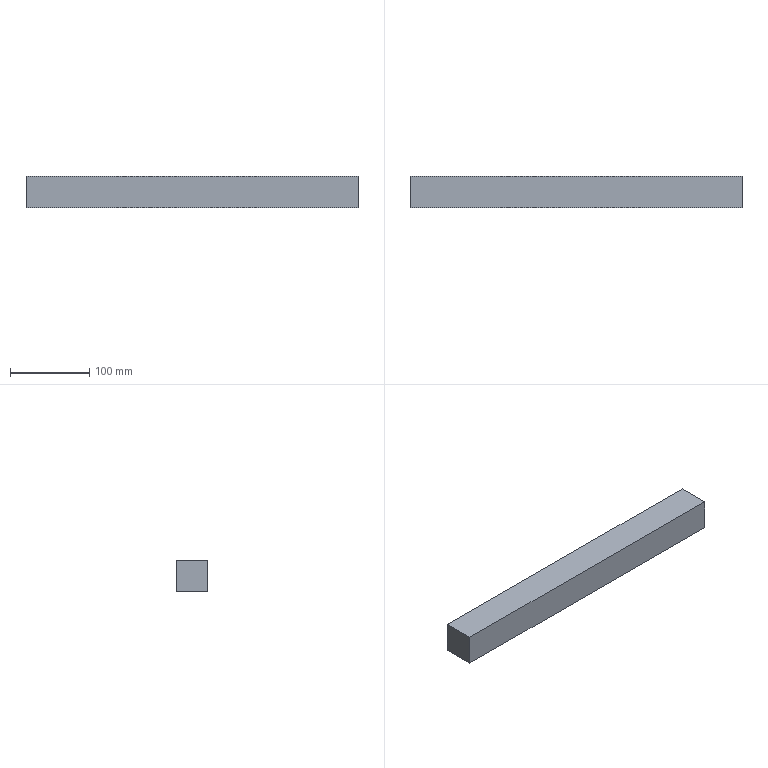Part | NX | 1 solid | 6 faces | box 420 x 40 x 40 mm | volume 672000 mm3 | plane 6
STEP:
#1=CARTESIAN_POINT('',(-369.726,88.985,0.));
#2=VERTEX_POINT('',#1);
#3=CARTESIAN_POINT('',(-369.726,88.985,-40.));
#4=VERTEX_POINT('',#3);
#5=CARTESIAN_POINT('',(-369.726,88.985,0.));
#6=DIRECTION('',(0.,0.,-1.));
#7=VECTOR('',#6,1000.);
#8=LINE('',#5,#7);
#9=EDGE_CURVE('',#2,#4,#8,.T.);
#10=ORIENTED_EDGE('',*,*,#9,.F.);
#11=CARTESIAN_POINT('',(50.274,88.985,0.));
#12=VERTEX_POINT('',#11);
#13=CARTESIAN_POINT('',(-369.726,88.985,0.));
#14=DIRECTION('',(1.,0.,0.));
#15=VECTOR('',#14,1000.);
#16=LINE('',#13,#15);
#17=EDGE_CURVE('',#2,#12,#16,.T.);
#18=ORIENTED_EDGE('',*,*,#17,.T.);
#19=CARTESIAN_POINT('',(50.274,88.985,-40.));
#20=VERTEX_POINT('',#19);
#21=CARTESIAN_POINT('',(50.274,88.985,0.));
#22=DIRECTION('',(0.,0.,-1.));
#23=VECTOR('',#22,1000.);
#24=LINE('',#21,#23);
#25=EDGE_CURVE('',#12,#20,#24,.T.);
#26=ORIENTED_EDGE('',*,*,#25,.T.);
#27=CARTESIAN_POINT('',(-369.726,88.985,-40.));
#28=DIRECTION('',(1.,0.,0.));
#29=VECTOR('',#28,1000.);
#30=LINE('',#27,#29);
#31=EDGE_CURVE('',#4,#20,#30,.T.);
#32=ORIENTED_EDGE('',*,*,#31,.F.);
#33=EDGE_LOOP('',(#10,#18,#26,#32));
#34=FACE_BOUND('',#33,.T.);
#35=CARTESIAN_POINT('',(-369.726,88.985,0.));
#36=DIRECTION('',(0.,1.,0.));
#37=DIRECTION('',(1.,0.,0.));
#38=AXIS2_PLACEMENT_3D('',#35,#36,#37);
#39=PLANE('',#38);
#40=ADVANCED_FACE('',(#34),#39,.T.);
#41=CARTESIAN_POINT('',(-369.726,48.985,0.));
#42=VERTEX_POINT('',#41);
#43=CARTESIAN_POINT('',(-369.726,88.985,0.));
#44=DIRECTION('',(0.,-1.,0.));
#45=VECTOR('',#44,1000.);
#46=LINE('',#43,#45);
#47=EDGE_CURVE('',#2,#42,#46,.T.);
#48=ORIENTED_EDGE('',*,*,#47,.T.);
#49=CARTESIAN_POINT('',(50.274,48.985,0.));
#50=VERTEX_POINT('',#49);
#51=CARTESIAN_POINT('',(-369.726,48.985,0.));
#52=DIRECTION('',(1.,0.,0.));
#53=VECTOR('',#52,1000.);
#54=LINE('',#51,#53);
#55=EDGE_CURVE('',#42,#50,#54,.T.);
#56=ORIENTED_EDGE('',*,*,#55,.T.);
#57=CARTESIAN_POINT('',(50.274,88.985,0.));
#58=DIRECTION('',(0.,-1.,0.));
#59=VECTOR('',#58,1000.);
#60=LINE('',#57,#59);
#61=EDGE_CURVE('',#12,#50,#60,.T.);
#62=ORIENTED_EDGE('',*,*,#61,.F.);
#63=ORIENTED_EDGE('',*,*,#17,.F.);
#64=EDGE_LOOP('',(#48,#56,#62,#63));
#65=FACE_BOUND('',#64,.T.);
#66=CARTESIAN_POINT('',(-369.726,48.985,0.));
#67=DIRECTION('',(0.,0.,1.));
#68=DIRECTION('',(1.,0.,0.));
#69=AXIS2_PLACEMENT_3D('',#66,#67,#68);
#70=PLANE('',#69);
#71=ADVANCED_FACE('',(#65),#70,.T.);
#72=CARTESIAN_POINT('',(-369.726,48.985,-40.));
#73=VERTEX_POINT('',#72);
#74=CARTESIAN_POINT('',(-369.726,48.985,0.));
#75=DIRECTION('',(0.,0.,-1.));
#76=VECTOR('',#75,1000.);
#77=LINE('',#74,#76);
#78=EDGE_CURVE('',#42,#73,#77,.T.);
#79=ORIENTED_EDGE('',*,*,#78,.T.);
#80=CARTESIAN_POINT('',(50.274,48.985,-40.));
#81=VERTEX_POINT('',#80);
#82=CARTESIAN_POINT('',(-369.726,48.985,-40.));
#83=DIRECTION('',(1.,0.,0.));
#84=VECTOR('',#83,1000.);
#85=LINE('',#82,#84);
#86=EDGE_CURVE('',#73,#81,#85,.T.);
#87=ORIENTED_EDGE('',*,*,#86,.T.);
#88=CARTESIAN_POINT('',(50.274,48.985,0.));
#89=DIRECTION('',(0.,0.,-1.));
#90=VECTOR('',#89,1000.);
#91=LINE('',#88,#90);
#92=EDGE_CURVE('',#50,#81,#91,.T.);
#93=ORIENTED_EDGE('',*,*,#92,.F.);
#94=ORIENTED_EDGE('',*,*,#55,.F.);
#95=EDGE_LOOP('',(#79,#87,#93,#94));
#96=FACE_BOUND('',#95,.T.);
#97=CARTESIAN_POINT('',(-369.726,48.985,-40.));
#98=DIRECTION('',(0.,-1.,0.));
#99=DIRECTION('',(0.,0.,-1.));
#100=AXIS2_PLACEMENT_3D('',#97,#98,#99);
#101=PLANE('',#100);
#102=ADVANCED_FACE('',(#96),#101,.T.);
#103=CARTESIAN_POINT('',(-369.726,88.985,-40.));
#104=DIRECTION('',(0.,-1.,0.));
#105=VECTOR('',#104,1000.);
#106=LINE('',#103,#105);
#107=EDGE_CURVE('',#4,#73,#106,.T.);
#108=ORIENTED_EDGE('',*,*,#107,.F.);
#109=ORIENTED_EDGE('',*,*,#31,.T.);
#110=CARTESIAN_POINT('',(50.274,88.985,-40.));
#111=DIRECTION('',(0.,-1.,0.));
#112=VECTOR('',#111,1000.);
#113=LINE('',#110,#112);
#114=EDGE_CURVE('',#20,#81,#113,.T.);
#115=ORIENTED_EDGE('',*,*,#114,.T.);
#116=ORIENTED_EDGE('',*,*,#86,.F.);
#117=EDGE_LOOP('',(#108,#109,#115,#116));
#118=FACE_BOUND('',#117,.T.);
#119=CARTESIAN_POINT('',(-369.726,88.985,-40.));
#120=DIRECTION('',(0.,0.,-1.));
#121=DIRECTION('',(0.,-1.,0.));
#122=AXIS2_PLACEMENT_3D('',#119,#120,#121);
#123=PLANE('',#122);
#124=ADVANCED_FACE('',(#118),#123,.T.);
#125=ORIENTED_EDGE('',*,*,#25,.F.);
#126=ORIENTED_EDGE('',*,*,#61,.T.);
#127=ORIENTED_EDGE('',*,*,#92,.T.);
#128=ORIENTED_EDGE('',*,*,#114,.F.);
#129=EDGE_LOOP('',(#125,#126,#127,#128));
#130=FACE_BOUND('',#129,.T.);
#131=CARTESIAN_POINT('',(50.274,64.663,-358.89));
#132=DIRECTION('',(1.,0.,0.));
#133=DIRECTION('',(0.,1.,0.));
#134=AXIS2_PLACEMENT_3D('',#131,#132,#133);
#135=PLANE('',#134);
#136=ADVANCED_FACE('',(#130),#135,.T.);
#137=ORIENTED_EDGE('',*,*,#107,.T.);
#138=ORIENTED_EDGE('',*,*,#78,.F.);
#139=ORIENTED_EDGE('',*,*,#47,.F.);
#140=ORIENTED_EDGE('',*,*,#9,.T.);
#141=EDGE_LOOP('',(#137,#138,#139,#140));
#142=FACE_BOUND('',#141,.T.);
#143=CARTESIAN_POINT('',(-369.726,64.663,-358.89));
#144=DIRECTION('',(1.,0.,0.));
#145=DIRECTION('',(0.,1.,0.));
#146=AXIS2_PLACEMENT_3D('',#143,#144,#145);
#147=PLANE('',#146);
#148=ADVANCED_FACE('',(#142),#147,.F.);
#149=CLOSED_SHELL('',(#40,#71,#102,#124,#136,#148));
#150=MANIFOLD_SOLID_BREP('',#149);
#151=(LENGTH_UNIT()NAMED_UNIT(*)SI_UNIT(.MILLI.,.METRE.));
#152=UNCERTAINTY_MEASURE_WITH_UNIT(LENGTH_MEASURE(0.00001),#151,'','');
#153=(NAMED_UNIT(*)PLANE_ANGLE_UNIT()SI_UNIT($,.RADIAN.));
#154=(NAMED_UNIT(*)SI_UNIT($,.STERADIAN.)SOLID_ANGLE_UNIT());
#155=(GEOMETRIC_REPRESENTATION_CONTEXT(3)GLOBAL_UNCERTAINTY_ASSIGNED_CONTEXT((#152))GLOBAL_UNIT_ASSIGNED_CONTEXT((#151,#153,#154))REPRESENTATION_CONTEXT('',''));
#156=ADVANCED_BREP_SHAPE_REPRESENTATION('',(#150),#155);